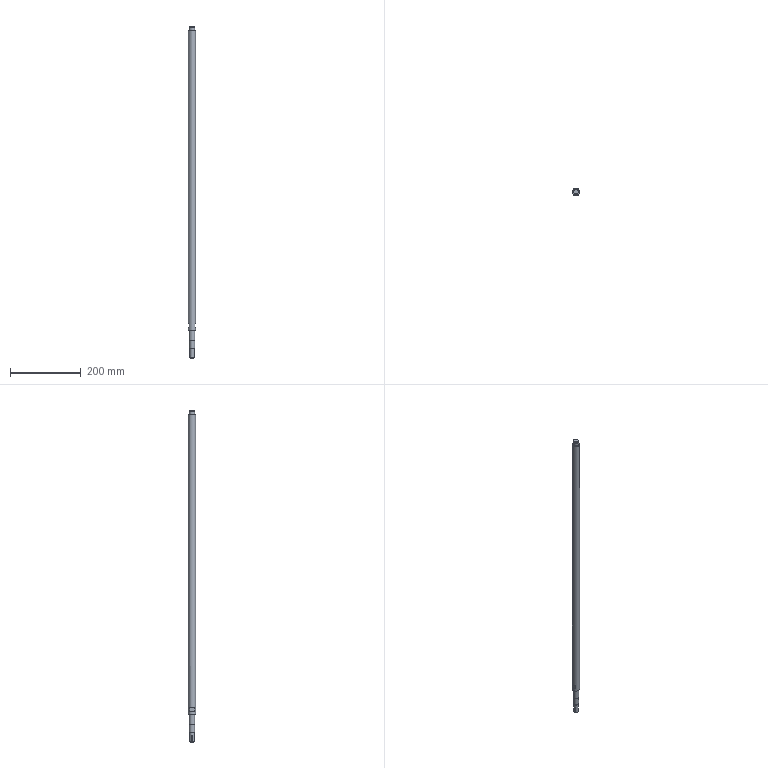Part | NX | 1 solid | 34 faces | box 20 x 20 x 936 mm | volume 278866 mm3 | plane 17 | cylinder 9 | cone 6 | torus 2 | commonest cylinder face diameters 15 x3 3.3 x1 4 x1 12 x1 14.3 x1 14.6 x1
STEP:
#1=CARTESIAN_POINT('',(7.5,0.,923.));
#2=VERTEX_POINT('',#1);
#3=CARTESIAN_POINT('',(0.,0.,923.));
#4=DIRECTION('',(0.,0.,1.));
#5=DIRECTION('',(1.,0.,0.));
#6=AXIS2_PLACEMENT_3D('',#3,#4,#5);
#7=CIRCLE('',#6,7.5);
#8=EDGE_CURVE('',#2,#2,#7,.T.);
#9=ORIENTED_EDGE('',*,*,#8,.T.);
#10=EDGE_LOOP('',(#9));
#11=FACE_BOUND('',#10,.T.);
#12=CARTESIAN_POINT('',(-7.5,0.,931.995));
#13=VERTEX_POINT('',#12);
#14=CARTESIAN_POINT('',(0.,0.,931.995));
#15=DIRECTION('',(0.,0.,-1.));
#16=DIRECTION('',(-1.,0.,0.));
#17=AXIS2_PLACEMENT_3D('',#14,#15,#16);
#18=CIRCLE('',#17,7.5);
#19=EDGE_CURVE('',#13,#13,#18,.T.);
#20=ORIENTED_EDGE('',*,*,#19,.T.);
#21=EDGE_LOOP('',(#20));
#22=FACE_BOUND('',#21,.T.);
#23=CARTESIAN_POINT('',(0.,0.,936.));
#24=DIRECTION('',(0.,0.,-1.));
#25=DIRECTION('',(-1.,0.,0.));
#26=AXIS2_PLACEMENT_3D('',#23,#24,#25);
#27=CYLINDRICAL_SURFACE('',#26,7.5);
#28=ADVANCED_FACE('',(#11,#22),#27,.T.);
#29=CARTESIAN_POINT('',(7.5,0.,78.));
#30=VERTEX_POINT('',#29);
#31=CARTESIAN_POINT('',(0.,0.,78.));
#32=DIRECTION('',(0.,0.,1.));
#33=DIRECTION('',(1.,0.,0.));
#34=AXIS2_PLACEMENT_3D('',#31,#32,#33);
#35=CIRCLE('',#34,7.5);
#36=EDGE_CURVE('',#30,#30,#35,.T.);
#37=ORIENTED_EDGE('',*,*,#36,.F.);
#38=EDGE_LOOP('',(#37));
#39=FACE_BOUND('',#38,.T.);
#40=CARTESIAN_POINT('',(-7.5,0.,50.));
#41=VERTEX_POINT('',#40);
#42=CARTESIAN_POINT('',(0.,0.,50.));
#43=DIRECTION('',(0.,0.,-1.));
#44=DIRECTION('',(-1.,0.,0.));
#45=AXIS2_PLACEMENT_3D('',#42,#43,#44);
#46=CIRCLE('',#45,7.5);
#47=EDGE_CURVE('',#41,#41,#46,.T.);
#48=ORIENTED_EDGE('',*,*,#47,.F.);
#49=EDGE_LOOP('',(#48));
#50=FACE_BOUND('',#49,.T.);
#51=CARTESIAN_POINT('',(0.,0.,78.));
#52=DIRECTION('',(0.,0.,-1.));
#53=DIRECTION('',(-1.,0.,0.));
#54=AXIS2_PLACEMENT_3D('',#51,#52,#53);
#55=CYLINDRICAL_SURFACE('',#54,7.5);
#56=ADVANCED_FACE('',(#39,#50),#55,.T.);
#57=CARTESIAN_POINT('',(10.,0.,922.7));
#58=VERTEX_POINT('',#57);
#59=CARTESIAN_POINT('',(0.,0.,922.7));
#60=DIRECTION('',(0.,0.,1.));
#61=DIRECTION('',(1.,0.,0.));
#62=AXIS2_PLACEMENT_3D('',#59,#60,#61);
#63=CIRCLE('',#62,10.);
#64=EDGE_CURVE('',#58,#58,#63,.F.);
#65=ORIENTED_EDGE('',*,*,#64,.T.);
#66=EDGE_LOOP('',(#65));
#67=FACE_BOUND('',#66,.T.);
#68=CARTESIAN_POINT('',(10.,0.,78.3));
#69=VERTEX_POINT('',#68);
#70=CARTESIAN_POINT('',(0.,0.,78.3));
#71=DIRECTION('',(0.,0.,1.));
#72=DIRECTION('',(1.,0.,0.));
#73=AXIS2_PLACEMENT_3D('',#70,#71,#72);
#74=CIRCLE('',#73,10.);
#75=EDGE_CURVE('',#69,#69,#74,.T.);
#76=ORIENTED_EDGE('',*,*,#75,.T.);
#77=EDGE_LOOP('',(#76));
#78=FACE_BOUND('',#77,.T.);
#79=CARTESIAN_POINT('',(-8.,-6.,97.));
#80=VERTEX_POINT('',#79);
#81=CARTESIAN_POINT('',(-8.,6.,97.));
#82=VERTEX_POINT('',#81);
#83=CARTESIAN_POINT('',(0.,0.,97.));
#84=DIRECTION('',(0.,0.,-1.));
#85=DIRECTION('',(-1.,0.,0.));
#86=AXIS2_PLACEMENT_3D('',#83,#84,#85);
#87=CIRCLE('',#86,10.);
#88=EDGE_CURVE('',#80,#82,#87,.T.);
#89=ORIENTED_EDGE('',*,*,#88,.F.);
#90=CARTESIAN_POINT('',(-8.,-6.,86.));
#91=VERTEX_POINT('',#90);
#92=CARTESIAN_POINT('',(-8.,-6.,923.));
#93=DIRECTION('',(0.,0.,-1.));
#94=VECTOR('',#93,1000.);
#95=LINE('',#92,#94);
#96=EDGE_CURVE('',#80,#91,#95,.T.);
#97=ORIENTED_EDGE('',*,*,#96,.T.);
#98=CARTESIAN_POINT('',(-8.,6.,86.));
#99=VERTEX_POINT('',#98);
#100=CARTESIAN_POINT('',(0.,0.,86.));
#101=DIRECTION('',(0.,0.,-1.));
#102=DIRECTION('',(-1.,0.,0.));
#103=AXIS2_PLACEMENT_3D('',#100,#101,#102);
#104=CIRCLE('',#103,10.);
#105=EDGE_CURVE('',#91,#99,#104,.T.);
#106=ORIENTED_EDGE('',*,*,#105,.T.);
#107=CARTESIAN_POINT('',(-8.,6.,923.));
#108=DIRECTION('',(0.,0.,-1.));
#109=VECTOR('',#108,1000.);
#110=LINE('',#107,#109);
#111=EDGE_CURVE('',#99,#82,#110,.F.);
#112=ORIENTED_EDGE('',*,*,#111,.T.);
#113=EDGE_LOOP('',(#89,#97,#106,#112));
#114=FACE_BOUND('',#113,.T.);
#115=CARTESIAN_POINT('',(8.,6.,97.));
#116=VERTEX_POINT('',#115);
#117=CARTESIAN_POINT('',(8.,-6.,97.));
#118=VERTEX_POINT('',#117);
#119=CARTESIAN_POINT('',(0.,0.,97.));
#120=DIRECTION('',(0.,0.,-1.));
#121=DIRECTION('',(-1.,0.,0.));
#122=AXIS2_PLACEMENT_3D('',#119,#120,#121);
#123=CIRCLE('',#122,10.);
#124=EDGE_CURVE('',#116,#118,#123,.T.);
#125=ORIENTED_EDGE('',*,*,#124,.F.);
#126=CARTESIAN_POINT('',(8.,6.,86.));
#127=VERTEX_POINT('',#126);
#128=CARTESIAN_POINT('',(8.,6.,923.));
#129=DIRECTION('',(0.,0.,-1.));
#130=VECTOR('',#129,1000.);
#131=LINE('',#128,#130);
#132=EDGE_CURVE('',#116,#127,#131,.T.);
#133=ORIENTED_EDGE('',*,*,#132,.T.);
#134=CARTESIAN_POINT('',(8.,-6.,86.));
#135=VERTEX_POINT('',#134);
#136=CARTESIAN_POINT('',(0.,0.,86.));
#137=DIRECTION('',(0.,0.,-1.));
#138=DIRECTION('',(-1.,0.,0.));
#139=AXIS2_PLACEMENT_3D('',#136,#137,#138);
#140=CIRCLE('',#139,10.);
#141=EDGE_CURVE('',#127,#135,#140,.T.);
#142=ORIENTED_EDGE('',*,*,#141,.T.);
#143=CARTESIAN_POINT('',(8.,-6.,923.));
#144=DIRECTION('',(0.,0.,-1.));
#145=VECTOR('',#144,1000.);
#146=LINE('',#143,#145);
#147=EDGE_CURVE('',#135,#118,#146,.F.);
#148=ORIENTED_EDGE('',*,*,#147,.T.);
#149=EDGE_LOOP('',(#125,#133,#142,#148));
#150=FACE_BOUND('',#149,.T.);
#151=CARTESIAN_POINT('',(0.,0.,923.));
#152=DIRECTION('',(0.,0.,-1.));
#153=DIRECTION('',(-1.,0.,0.));
#154=AXIS2_PLACEMENT_3D('',#151,#152,#153);
#155=CYLINDRICAL_SURFACE('',#154,10.);
#156=ADVANCED_FACE('',(#67,#78,#114,#150),#155,.T.);
#157=CARTESIAN_POINT('',(9.7,0.,923.));
#158=VERTEX_POINT('',#157);
#159=CARTESIAN_POINT('',(0.,0.,923.));
#160=DIRECTION('',(0.,0.,1.));
#161=DIRECTION('',(1.,0.,0.));
#162=AXIS2_PLACEMENT_3D('',#159,#160,#161);
#163=CIRCLE('',#162,9.7);
#164=EDGE_CURVE('',#158,#158,#163,.T.);
#165=ORIENTED_EDGE('',*,*,#164,.T.);
#166=EDGE_LOOP('',(#165));
#167=FACE_BOUND('',#166,.T.);
#168=ORIENTED_EDGE('',*,*,#8,.F.);
#169=EDGE_LOOP('',(#168));
#170=FACE_BOUND('',#169,.T.);
#171=CARTESIAN_POINT('',(0.,0.,923.));
#172=DIRECTION('',(0.,0.,1.));
#173=DIRECTION('',(1.,0.,0.));
#174=AXIS2_PLACEMENT_3D('',#171,#172,#173);
#175=PLANE('',#174);
#176=ADVANCED_FACE('',(#167,#170),#175,.T.);
#177=CARTESIAN_POINT('',(9.7,0.,78.));
#178=VERTEX_POINT('',#177);
#179=CARTESIAN_POINT('',(0.,0.,78.));
#180=DIRECTION('',(0.,0.,1.));
#181=DIRECTION('',(1.,0.,0.));
#182=AXIS2_PLACEMENT_3D('',#179,#180,#181);
#183=CIRCLE('',#182,9.7);
#184=EDGE_CURVE('',#178,#178,#183,.F.);
#185=ORIENTED_EDGE('',*,*,#184,.T.);
#186=EDGE_LOOP('',(#185));
#187=FACE_BOUND('',#186,.T.);
#188=ORIENTED_EDGE('',*,*,#36,.T.);
#189=EDGE_LOOP('',(#188));
#190=FACE_BOUND('',#189,.T.);
#191=CARTESIAN_POINT('',(0.,0.,78.));
#192=DIRECTION('',(0.,0.,1.));
#193=DIRECTION('',(1.,0.,0.));
#194=AXIS2_PLACEMENT_3D('',#191,#192,#193);
#195=PLANE('',#194);
#196=ADVANCED_FACE('',(#187,#190),#195,.F.);
#197=CARTESIAN_POINT('',(-8.,20.,97.));
#198=DIRECTION('',(0.,-1.,0.));
#199=VECTOR('',#198,1000.);
#200=LINE('',#197,#199);
#201=EDGE_CURVE('',#82,#80,#200,.T.);
#202=ORIENTED_EDGE('',*,*,#201,.F.);
#203=ORIENTED_EDGE('',*,*,#111,.F.);
#204=CARTESIAN_POINT('',(-8.,20.,86.));
#205=DIRECTION('',(0.,-1.,0.));
#206=VECTOR('',#205,1000.);
#207=LINE('',#204,#206);
#208=EDGE_CURVE('',#99,#91,#207,.T.);
#209=ORIENTED_EDGE('',*,*,#208,.T.);
#210=ORIENTED_EDGE('',*,*,#96,.F.);
#211=EDGE_LOOP('',(#202,#203,#209,#210));
#212=FACE_BOUND('',#211,.T.);
#213=CARTESIAN_POINT('',(-8.,20.,97.));
#214=DIRECTION('',(1.,0.,0.));
#215=DIRECTION('',(0.,0.,-1.));
#216=AXIS2_PLACEMENT_3D('',#213,#214,#215);
#217=PLANE('',#216);
#218=ADVANCED_FACE('',(#212),#217,.F.);
#219=ORIENTED_EDGE('',*,*,#88,.T.);
#220=ORIENTED_EDGE('',*,*,#201,.T.);
#221=EDGE_LOOP('',(#219,#220));
#222=FACE_BOUND('',#221,.T.);
#223=CARTESIAN_POINT('',(-20.,-20.,97.));
#224=DIRECTION('',(0.,0.,-1.));
#225=DIRECTION('',(-1.,0.,0.));
#226=AXIS2_PLACEMENT_3D('',#223,#224,#225);
#227=PLANE('',#226);
#228=ADVANCED_FACE('',(#222),#227,.T.);
#229=ORIENTED_EDGE('',*,*,#208,.F.);
#230=ORIENTED_EDGE('',*,*,#105,.F.);
#231=EDGE_LOOP('',(#229,#230));
#232=FACE_BOUND('',#231,.T.);
#233=CARTESIAN_POINT('',(-20.,-20.,86.));
#234=DIRECTION('',(0.,0.,-1.));
#235=DIRECTION('',(-1.,0.,0.));
#236=AXIS2_PLACEMENT_3D('',#233,#234,#235);
#237=PLANE('',#236);
#238=ADVANCED_FACE('',(#232),#237,.F.);
#239=CARTESIAN_POINT('',(8.,20.,97.));
#240=DIRECTION('',(0.,1.,0.));
#241=VECTOR('',#240,1000.);
#242=LINE('',#239,#241);
#243=EDGE_CURVE('',#118,#116,#242,.T.);
#244=ORIENTED_EDGE('',*,*,#243,.F.);
#245=ORIENTED_EDGE('',*,*,#147,.F.);
#246=CARTESIAN_POINT('',(8.,20.,86.));
#247=DIRECTION('',(0.,1.,0.));
#248=VECTOR('',#247,1000.);
#249=LINE('',#246,#248);
#250=EDGE_CURVE('',#135,#127,#249,.T.);
#251=ORIENTED_EDGE('',*,*,#250,.T.);
#252=ORIENTED_EDGE('',*,*,#132,.F.);
#253=EDGE_LOOP('',(#244,#245,#251,#252));
#254=FACE_BOUND('',#253,.T.);
#255=CARTESIAN_POINT('',(8.,20.,97.));
#256=DIRECTION('',(-1.,0.,0.));
#257=DIRECTION('',(0.,0.,1.));
#258=AXIS2_PLACEMENT_3D('',#255,#256,#257);
#259=PLANE('',#258);
#260=ADVANCED_FACE('',(#254),#259,.F.);
#261=ORIENTED_EDGE('',*,*,#124,.T.);
#262=ORIENTED_EDGE('',*,*,#243,.T.);
#263=EDGE_LOOP('',(#261,#262));
#264=FACE_BOUND('',#263,.T.);
#265=CARTESIAN_POINT('',(8.,-20.,97.));
#266=DIRECTION('',(0.,0.,-1.));
#267=DIRECTION('',(-1.,0.,0.));
#268=AXIS2_PLACEMENT_3D('',#265,#266,#267);
#269=PLANE('',#268);
#270=ADVANCED_FACE('',(#264),#269,.T.);
#271=ORIENTED_EDGE('',*,*,#250,.F.);
#272=ORIENTED_EDGE('',*,*,#141,.F.);
#273=EDGE_LOOP('',(#271,#272));
#274=FACE_BOUND('',#273,.T.);
#275=CARTESIAN_POINT('',(8.,-20.,86.));
#276=DIRECTION('',(0.,0.,-1.));
#277=DIRECTION('',(-1.,0.,0.));
#278=AXIS2_PLACEMENT_3D('',#275,#276,#277);
#279=PLANE('',#278);
#280=ADVANCED_FACE('',(#274),#279,.F.);
#281=ORIENTED_EDGE('',*,*,#64,.F.);
#282=EDGE_LOOP('',(#281));
#283=FACE_BOUND('',#282,.T.);
#284=ORIENTED_EDGE('',*,*,#164,.F.);
#285=EDGE_LOOP('',(#284));
#286=FACE_BOUND('',#285,.T.);
#287=CARTESIAN_POINT('',(0.,0.,923.));
#288=DIRECTION('',(0.,0.,-1.));
#289=DIRECTION('',(-1.,0.,0.));
#290=AXIS2_PLACEMENT_3D('',#287,#288,#289);
#291=CONICAL_SURFACE('',#290,9.7,0.7854);
#292=ADVANCED_FACE('',(#283,#286),#291,.T.);
#293=ORIENTED_EDGE('',*,*,#184,.F.);
#294=EDGE_LOOP('',(#293));
#295=FACE_BOUND('',#294,.T.);
#296=ORIENTED_EDGE('',*,*,#75,.F.);
#297=EDGE_LOOP('',(#296));
#298=FACE_BOUND('',#297,.T.);
#299=CARTESIAN_POINT('',(0.,0.,78.3));
#300=DIRECTION('',(0.,0.,1.));
#301=DIRECTION('',(1.,0.,0.));
#302=AXIS2_PLACEMENT_3D('',#299,#300,#301);
#303=CONICAL_SURFACE('',#302,10.,0.7854);
#304=ADVANCED_FACE('',(#295,#298),#303,.T.);
#305=CARTESIAN_POINT('',(-7.3,0.,50.));
#306=VERTEX_POINT('',#305);
#307=CARTESIAN_POINT('',(0.,0.,50.));
#308=DIRECTION('',(0.,0.,-1.));
#309=DIRECTION('',(-1.,0.,0.));
#310=AXIS2_PLACEMENT_3D('',#307,#308,#309);
#311=CIRCLE('',#310,7.3);
#312=EDGE_CURVE('',#306,#306,#311,.T.);
#313=ORIENTED_EDGE('',*,*,#312,.F.);
#314=EDGE_LOOP('',(#313));
#315=FACE_BOUND('',#314,.T.);
#316=ORIENTED_EDGE('',*,*,#47,.T.);
#317=EDGE_LOOP('',(#316));
#318=FACE_BOUND('',#317,.T.);
#319=CARTESIAN_POINT('',(0.,0.,50.));
#320=DIRECTION('',(0.,0.,-1.));
#321=DIRECTION('',(-1.,0.,0.));
#322=AXIS2_PLACEMENT_3D('',#319,#320,#321);
#323=PLANE('',#322);
#324=ADVANCED_FACE('',(#315,#318),#323,.T.);
#325=CARTESIAN_POINT('',(7.3,0.,28.1));
#326=VERTEX_POINT('',#325);
#327=CARTESIAN_POINT('',(0.,0.,28.1));
#328=DIRECTION('',(0.,0.,1.));
#329=DIRECTION('',(1.,0.,0.));
#330=AXIS2_PLACEMENT_3D('',#327,#328,#329);
#331=CIRCLE('',#330,7.3);
#332=EDGE_CURVE('',#326,#326,#331,.F.);
#333=ORIENTED_EDGE('',*,*,#332,.F.);
#334=EDGE_LOOP('',(#333));
#335=FACE_BOUND('',#334,.T.);
#336=ORIENTED_EDGE('',*,*,#312,.T.);
#337=EDGE_LOOP('',(#336));
#338=FACE_BOUND('',#337,.T.);
#339=CARTESIAN_POINT('',(0.,0.,50.));
#340=DIRECTION('',(0.,0.,-1.));
#341=DIRECTION('',(-1.,0.,0.));
#342=AXIS2_PLACEMENT_3D('',#339,#340,#341);
#343=CYLINDRICAL_SURFACE('',#342,7.3);
#344=ADVANCED_FACE('',(#335,#338),#343,.T.);
#345=CARTESIAN_POINT('',(-1.65,0.,0.));
#346=VERTEX_POINT('',#345);
#347=CARTESIAN_POINT('',(0.,0.,0.));
#348=DIRECTION('',(0.,0.,-1.));
#349=DIRECTION('',(-1.,0.,0.));
#350=AXIS2_PLACEMENT_3D('',#347,#348,#349);
#351=CIRCLE('',#350,1.65);
#352=EDGE_CURVE('',#346,#346,#351,.T.);
#353=ORIENTED_EDGE('',*,*,#352,.F.);
#354=EDGE_LOOP('',(#353));
#355=FACE_BOUND('',#354,.T.);
#356=CARTESIAN_POINT('',(-3.5,2.,0.));
#357=VERTEX_POINT('',#356);
#358=CARTESIAN_POINT('',(-3.5,-2.,0.));
#359=VERTEX_POINT('',#358);
#360=CARTESIAN_POINT('',(-3.5,0.,0.));
#361=DIRECTION('',(0.,-1.,0.));
#362=VECTOR('',#361,1000.);
#363=LINE('',#360,#362);
#364=EDGE_CURVE('',#357,#359,#363,.T.);
#365=ORIENTED_EDGE('',*,*,#364,.F.);
#366=CARTESIAN_POINT('',(-4.583,2.,0.));
#367=VERTEX_POINT('',#366);
#368=CARTESIAN_POINT('',(-3.5,2.,0.));
#369=DIRECTION('',(-1.,0.,0.));
#370=VECTOR('',#369,1000.);
#371=LINE('',#368,#370);
#372=EDGE_CURVE('',#357,#367,#371,.T.);
#373=ORIENTED_EDGE('',*,*,#372,.T.);
#374=CARTESIAN_POINT('',(-4.583,-2.,0.));
#375=VERTEX_POINT('',#374);
#376=CARTESIAN_POINT('',(0.,0.,0.));
#377=DIRECTION('',(0.,0.,1.));
#378=DIRECTION('',(1.,0.,0.));
#379=AXIS2_PLACEMENT_3D('',#376,#377,#378);
#380=CIRCLE('',#379,5.);
#381=EDGE_CURVE('',#367,#375,#380,.F.);
#382=ORIENTED_EDGE('',*,*,#381,.T.);
#383=CARTESIAN_POINT('',(-3.5,-2.,0.));
#384=DIRECTION('',(-1.,0.,0.));
#385=VECTOR('',#384,1000.);
#386=LINE('',#383,#385);
#387=EDGE_CURVE('',#359,#375,#386,.T.);
#388=ORIENTED_EDGE('',*,*,#387,.F.);
#389=EDGE_LOOP('',(#365,#373,#382,#388));
#390=FACE_BOUND('',#389,.T.);
#391=CARTESIAN_POINT('',(0.,0.,0.));
#392=DIRECTION('',(0.,0.,1.));
#393=DIRECTION('',(1.,0.,0.));
#394=AXIS2_PLACEMENT_3D('',#391,#392,#393);
#395=PLANE('',#394);
#396=ADVANCED_FACE('',(#355,#390),#395,.F.);
#397=CARTESIAN_POINT('',(-5.657,-2.,1.));
#398=VERTEX_POINT('',#397);
#399=CARTESIAN_POINT('',(-5.657,2.,1.));
#400=VERTEX_POINT('',#399);
#401=CARTESIAN_POINT('',(0.,0.,1.));
#402=DIRECTION('',(0.,0.,1.));
#403=DIRECTION('',(1.,0.,0.));
#404=AXIS2_PLACEMENT_3D('',#401,#402,#403);
#405=CIRCLE('',#404,6.);
#406=EDGE_CURVE('',#398,#400,#405,.T.);
#407=ORIENTED_EDGE('',*,*,#406,.T.);
#408=CARTESIAN_POINT('',(-5.657,2.,16.));
#409=VERTEX_POINT('',#408);
#410=CARTESIAN_POINT('',(-5.657,2.,28.));
#411=DIRECTION('',(0.,0.,-1.));
#412=VECTOR('',#411,1000.);
#413=LINE('',#410,#412);
#414=EDGE_CURVE('',#400,#409,#413,.F.);
#415=ORIENTED_EDGE('',*,*,#414,.T.);
#416=CARTESIAN_POINT('',(-5.657,-2.,16.));
#417=VERTEX_POINT('',#416);
#418=CARTESIAN_POINT('',(-5.657,2.,16.));
#419=CARTESIAN_POINT('',(-5.657,2.,16.533));
#420=CARTESIAN_POINT('',(-5.833,1.567,17.562));
#421=CARTESIAN_POINT('',(-6.083,0.003461,18.219));
#422=CARTESIAN_POINT('',(-5.834,-1.568,17.563));
#423=CARTESIAN_POINT('',(-5.657,-2.,16.533));
#424=CARTESIAN_POINT('',(-5.657,-2.,16.));
#425=B_SPLINE_CURVE_WITH_KNOTS('',3,(#418,#419,#420,#421,#422,#423,#424),.UNSPECIFIED.,.F.,.F.,(4,1,1,1,4),(0.,0.001574,0.003148,0.004722,0.006296),.UNSPECIFIED.);
#426=EDGE_CURVE('',#409,#417,#425,.T.);
#427=ORIENTED_EDGE('',*,*,#426,.T.);
#428=CARTESIAN_POINT('',(-5.657,-2.,28.));
#429=DIRECTION('',(0.,0.,-1.));
#430=VECTOR('',#429,1000.);
#431=LINE('',#428,#430);
#432=EDGE_CURVE('',#417,#398,#431,.T.);
#433=ORIENTED_EDGE('',*,*,#432,.T.);
#434=EDGE_LOOP('',(#407,#415,#427,#433));
#435=FACE_BOUND('',#434,.T.);
#436=CARTESIAN_POINT('',(6.,0.,28.));
#437=VERTEX_POINT('',#436);
#438=CARTESIAN_POINT('',(0.,0.,28.));
#439=DIRECTION('',(0.,0.,1.));
#440=DIRECTION('',(1.,0.,0.));
#441=AXIS2_PLACEMENT_3D('',#438,#439,#440);
#442=CIRCLE('',#441,6.);
#443=EDGE_CURVE('',#437,#437,#442,.T.);
#444=ORIENTED_EDGE('',*,*,#443,.F.);
#445=EDGE_LOOP('',(#444));
#446=FACE_BOUND('',#445,.T.);
#447=CARTESIAN_POINT('',(0.,0.,28.));
#448=DIRECTION('',(0.,0.,-1.));
#449=DIRECTION('',(-1.,0.,0.));
#450=AXIS2_PLACEMENT_3D('',#447,#448,#449);
#451=CYLINDRICAL_SURFACE('',#450,6.);
#452=ADVANCED_FACE('',(#435,#446),#451,.T.);
#453=CARTESIAN_POINT('',(7.2,0.,28.));
#454=VERTEX_POINT('',#453);
#455=CARTESIAN_POINT('',(0.,0.,28.));
#456=DIRECTION('',(0.,0.,1.));
#457=DIRECTION('',(1.,0.,0.));
#458=AXIS2_PLACEMENT_3D('',#455,#456,#457);
#459=CIRCLE('',#458,7.2);
#460=EDGE_CURVE('',#454,#454,#459,.F.);
#461=ORIENTED_EDGE('',*,*,#460,.T.);
#462=EDGE_LOOP('',(#461));
#463=FACE_BOUND('',#462,.T.);
#464=ORIENTED_EDGE('',*,*,#443,.T.);
#465=EDGE_LOOP('',(#464));
#466=FACE_BOUND('',#465,.T.);
#467=CARTESIAN_POINT('',(0.,0.,28.));
#468=DIRECTION('',(0.,0.,1.));
#469=DIRECTION('',(1.,0.,0.));
#470=AXIS2_PLACEMENT_3D('',#467,#468,#469);
#471=PLANE('',#470);
#472=ADVANCED_FACE('',(#463,#466),#471,.F.);
#473=ORIENTED_EDGE('',*,*,#460,.F.);
#474=EDGE_LOOP('',(#473));
#475=FACE_BOUND('',#474,.T.);
#476=ORIENTED_EDGE('',*,*,#332,.T.);
#477=EDGE_LOOP('',(#476));
#478=FACE_BOUND('',#477,.T.);
#479=CARTESIAN_POINT('',(0.,0.,28.3));
#480=DIRECTION('',(0.,0.,1.));
#481=DIRECTION('',(1.,0.,0.));
#482=AXIS2_PLACEMENT_3D('',#479,#480,#481);
#483=CONICAL_SURFACE('',#482,7.5,0.7854);
#484=ADVANCED_FACE('',(#475,#478),#483,.T.);
#485=CARTESIAN_POINT('',(-7.5,0.,933.145));
#486=VERTEX_POINT('',#485);
#487=CARTESIAN_POINT('',(0.,0.,933.145));
#488=DIRECTION('',(0.,0.,-1.));
#489=DIRECTION('',(-1.,0.,0.));
#490=AXIS2_PLACEMENT_3D('',#487,#488,#489);
#491=CIRCLE('',#490,7.5);
#492=EDGE_CURVE('',#486,#486,#491,.T.);
#493=ORIENTED_EDGE('',*,*,#492,.T.);
#494=EDGE_LOOP('',(#493));
#495=FACE_BOUND('',#494,.T.);
#496=CARTESIAN_POINT('',(-7.26,0.,933.145));
#497=VERTEX_POINT('',#496);
#498=CARTESIAN_POINT('',(0.,0.,933.145));
#499=DIRECTION('',(0.,0.,-1.));
#500=DIRECTION('',(-1.,0.,0.));
#501=AXIS2_PLACEMENT_3D('',#498,#499,#500);
#502=CIRCLE('',#501,7.26);
#503=EDGE_CURVE('',#497,#497,#502,.T.);
#504=ORIENTED_EDGE('',*,*,#503,.F.);
#505=EDGE_LOOP('',(#504));
#506=FACE_BOUND('',#505,.T.);
#507=CARTESIAN_POINT('',(-7.26,-0.05092,933.145));
#508=DIRECTION('',(0.,0.,-1.));
#509=DIRECTION('',(-1.,0.,0.));
#510=AXIS2_PLACEMENT_3D('',#507,#508,#509);
#511=PLANE('',#510);
#512=ADVANCED_FACE('',(#495,#506),#511,.T.);
#513=ORIENTED_EDGE('',*,*,#503,.T.);
#514=EDGE_LOOP('',(#513));
#515=FACE_BOUND('',#514,.T.);
#516=CARTESIAN_POINT('',(-7.15,0.,933.035));
#517=VERTEX_POINT('',#516);
#518=CARTESIAN_POINT('',(0.,0.,933.035));
#519=DIRECTION('',(0.,0.,-1.));
#520=DIRECTION('',(-1.,0.,0.));
#521=AXIS2_PLACEMENT_3D('',#518,#519,#520);
#522=CIRCLE('',#521,7.15);
#523=EDGE_CURVE('',#517,#517,#522,.T.);
#524=ORIENTED_EDGE('',*,*,#523,.F.);
#525=EDGE_LOOP('',(#524));
#526=FACE_BOUND('',#525,.T.);
#527=CARTESIAN_POINT('',(0.,0.,933.035));
#528=DIRECTION('',(0.,0.,-1.));
#529=DIRECTION('',(-1.,0.,0.));
#530=AXIS2_PLACEMENT_3D('',#527,#528,#529);
#531=TOROIDAL_SURFACE('',#530,7.26,0.11);
#532=ADVANCED_FACE('',(#515,#526),#531,.F.);
#533=ORIENTED_EDGE('',*,*,#523,.T.);
#534=EDGE_LOOP('',(#533));
#535=FACE_BOUND('',#534,.T.);
#536=CARTESIAN_POINT('',(-7.15,0.,932.105));
#537=VERTEX_POINT('',#536);
#538=CARTESIAN_POINT('',(0.,0.,932.105));
#539=DIRECTION('',(0.,0.,-1.));
#540=DIRECTION('',(-1.,0.,0.));
#541=AXIS2_PLACEMENT_3D('',#538,#539,#540);
#542=CIRCLE('',#541,7.15);
#543=EDGE_CURVE('',#537,#537,#542,.T.);
#544=ORIENTED_EDGE('',*,*,#543,.F.);
#545=EDGE_LOOP('',(#544));
#546=FACE_BOUND('',#545,.T.);
#547=CARTESIAN_POINT('',(0.,0.,1053.848));
#548=DIRECTION('',(0.,0.,-1.));
#549=DIRECTION('',(-1.,0.,0.));
#550=AXIS2_PLACEMENT_3D('',#547,#548,#549);
#551=CYLINDRICAL_SURFACE('',#550,7.15);
#552=ADVANCED_FACE('',(#535,#546),#551,.T.);
#553=ORIENTED_EDGE('',*,*,#543,.T.);
#554=EDGE_LOOP('',(#553));
#555=FACE_BOUND('',#554,.T.);
#556=CARTESIAN_POINT('',(-7.26,0.,931.995));
#557=VERTEX_POINT('',#556);
#558=CARTESIAN_POINT('',(0.,0.,931.995));
#559=DIRECTION('',(0.,0.,-1.));
#560=DIRECTION('',(-1.,0.,0.));
#561=AXIS2_PLACEMENT_3D('',#558,#559,#560);
#562=CIRCLE('',#561,7.26);
#563=EDGE_CURVE('',#557,#557,#562,.T.);
#564=ORIENTED_EDGE('',*,*,#563,.F.);
#565=EDGE_LOOP('',(#564));
#566=FACE_BOUND('',#565,.T.);
#567=CARTESIAN_POINT('',(0.,0.,932.105));
#568=DIRECTION('',(0.,0.,-1.));
#569=DIRECTION('',(-1.,0.,0.));
#570=AXIS2_PLACEMENT_3D('',#567,#568,#569);
#571=TOROIDAL_SURFACE('',#570,7.26,0.11);
#572=ADVANCED_FACE('',(#555,#566),#571,.F.);
#573=ORIENTED_EDGE('',*,*,#563,.T.);
#574=EDGE_LOOP('',(#573));
#575=FACE_BOUND('',#574,.T.);
#576=ORIENTED_EDGE('',*,*,#19,.F.);
#577=EDGE_LOOP('',(#576));
#578=FACE_BOUND('',#577,.T.);
#579=CARTESIAN_POINT('',(-7.5,-0.0526,931.995));
#580=DIRECTION('',(0.,0.,1.));
#581=DIRECTION('',(1.,0.,0.));
#582=AXIS2_PLACEMENT_3D('',#579,#580,#581);
#583=PLANE('',#582);
#584=ADVANCED_FACE('',(#575,#578),#583,.T.);
#585=CARTESIAN_POINT('',(6.5,0.,936.));
#586=VERTEX_POINT('',#585);
#587=CARTESIAN_POINT('',(0.,0.,936.));
#588=DIRECTION('',(0.,0.,1.));
#589=DIRECTION('',(1.,0.,0.));
#590=AXIS2_PLACEMENT_3D('',#587,#588,#589);
#591=CIRCLE('',#590,6.5);
#592=EDGE_CURVE('',#586,#586,#591,.T.);
#593=ORIENTED_EDGE('',*,*,#592,.T.);
#594=EDGE_LOOP('',(#593));
#595=FACE_BOUND('',#594,.T.);
#596=CARTESIAN_POINT('',(0.,0.,936.));
#597=DIRECTION('',(0.,0.,1.));
#598=DIRECTION('',(1.,0.,0.));
#599=AXIS2_PLACEMENT_3D('',#596,#597,#598);
#600=PLANE('',#599);
#601=ADVANCED_FACE('',(#595),#600,.T.);
#602=CARTESIAN_POINT('',(7.5,0.,935.));
#603=VERTEX_POINT('',#602);
#604=CARTESIAN_POINT('',(0.,0.,935.));
#605=DIRECTION('',(0.,0.,1.));
#606=DIRECTION('',(1.,0.,0.));
#607=AXIS2_PLACEMENT_3D('',#604,#605,#606);
#608=CIRCLE('',#607,7.5);
#609=EDGE_CURVE('',#603,#603,#608,.F.);
#610=ORIENTED_EDGE('',*,*,#609,.T.);
#611=EDGE_LOOP('',(#610));
#612=FACE_BOUND('',#611,.T.);
#613=ORIENTED_EDGE('',*,*,#492,.F.);
#614=EDGE_LOOP('',(#613));
#615=FACE_BOUND('',#614,.T.);
#616=CARTESIAN_POINT('',(0.,0.,936.));
#617=DIRECTION('',(0.,0.,-1.));
#618=DIRECTION('',(-1.,0.,0.));
#619=AXIS2_PLACEMENT_3D('',#616,#617,#618);
#620=CYLINDRICAL_SURFACE('',#619,7.5);
#621=ADVANCED_FACE('',(#612,#615),#620,.T.);
#622=ORIENTED_EDGE('',*,*,#609,.F.);
#623=EDGE_LOOP('',(#622));
#624=FACE_BOUND('',#623,.T.);
#625=ORIENTED_EDGE('',*,*,#592,.F.);
#626=EDGE_LOOP('',(#625));
#627=FACE_BOUND('',#626,.T.);
#628=CARTESIAN_POINT('',(0.,0.,936.));
#629=DIRECTION('',(0.,0.,-1.));
#630=DIRECTION('',(-1.,0.,0.));
#631=AXIS2_PLACEMENT_3D('',#628,#629,#630);
#632=CONICAL_SURFACE('',#631,6.5,0.7854);
#633=ADVANCED_FACE('',(#624,#627),#632,.T.);
#634=CARTESIAN_POINT('',(-5.657,2.,1.));
#635=CARTESIAN_POINT('',(-5.301,2.,0.6643));
#636=CARTESIAN_POINT('',(-4.943,2.,0.3304));
#637=CARTESIAN_POINT('',(-4.583,2.,0.));
#638=B_SPLINE_CURVE_WITH_KNOTS('',3,(#634,#635,#636,#637),.UNSPECIFIED.,.F.,.F.,(4,4),(0.005088,0.006556),.UNSPECIFIED.);
#639=EDGE_CURVE('',#400,#367,#638,.T.);
#640=ORIENTED_EDGE('',*,*,#639,.F.);
#641=ORIENTED_EDGE('',*,*,#406,.F.);
#642=CARTESIAN_POINT('',(-4.583,-2.,0.));
#643=CARTESIAN_POINT('',(-4.943,-2.,0.3305));
#644=CARTESIAN_POINT('',(-5.301,-2.,0.6644));
#645=CARTESIAN_POINT('',(-5.657,-2.,1.));
#646=B_SPLINE_CURVE_WITH_KNOTS('',3,(#642,#643,#644,#645),.UNSPECIFIED.,.F.,.F.,(4,4),(0.004277,0.005741),.UNSPECIFIED.);
#647=EDGE_CURVE('',#375,#398,#646,.T.);
#648=ORIENTED_EDGE('',*,*,#647,.F.);
#649=ORIENTED_EDGE('',*,*,#381,.F.);
#650=EDGE_LOOP('',(#640,#641,#648,#649));
#651=FACE_BOUND('',#650,.T.);
#652=CARTESIAN_POINT('',(0.,0.,1.));
#653=DIRECTION('',(0.,0.,1.));
#654=DIRECTION('',(1.,0.,0.));
#655=AXIS2_PLACEMENT_3D('',#652,#653,#654);
#656=CONICAL_SURFACE('',#655,6.,0.7854);
#657=ADVANCED_FACE('',(#651),#656,.T.);
#658=ORIENTED_EDGE('',*,*,#364,.T.);
#659=CARTESIAN_POINT('',(-3.5,-2.,16.));
#660=VERTEX_POINT('',#659);
#661=CARTESIAN_POINT('',(-3.5,-2.,0.));
#662=DIRECTION('',(0.,0.,1.));
#663=VECTOR('',#662,1000.);
#664=LINE('',#661,#663);
#665=EDGE_CURVE('',#359,#660,#664,.T.);
#666=ORIENTED_EDGE('',*,*,#665,.T.);
#667=CARTESIAN_POINT('',(-3.5,2.,16.));
#668=VERTEX_POINT('',#667);
#669=CARTESIAN_POINT('',(-3.5,0.,16.));
#670=DIRECTION('',(-1.,0.,0.));
#671=DIRECTION('',(0.,0.,1.));
#672=AXIS2_PLACEMENT_3D('',#669,#670,#671);
#673=CIRCLE('',#672,2.);
#674=EDGE_CURVE('',#660,#668,#673,.T.);
#675=ORIENTED_EDGE('',*,*,#674,.T.);
#676=CARTESIAN_POINT('',(-3.5,2.,0.));
#677=DIRECTION('',(0.,0.,-1.));
#678=VECTOR('',#677,1000.);
#679=LINE('',#676,#678);
#680=EDGE_CURVE('',#668,#357,#679,.T.);
#681=ORIENTED_EDGE('',*,*,#680,.T.);
#682=EDGE_LOOP('',(#658,#666,#675,#681));
#683=FACE_BOUND('',#682,.T.);
#684=CARTESIAN_POINT('',(-3.5,0.,0.));
#685=DIRECTION('',(-1.,0.,0.));
#686=DIRECTION('',(0.,0.,1.));
#687=AXIS2_PLACEMENT_3D('',#684,#685,#686);
#688=PLANE('',#687);
#689=ADVANCED_FACE('',(#683),#688,.T.);
#690=CARTESIAN_POINT('',(-3.5,2.,16.));
#691=DIRECTION('',(-1.,0.,0.));
#692=VECTOR('',#691,1000.);
#693=LINE('',#690,#692);
#694=EDGE_CURVE('',#668,#409,#693,.T.);
#695=ORIENTED_EDGE('',*,*,#694,.F.);
#696=ORIENTED_EDGE('',*,*,#674,.F.);
#697=CARTESIAN_POINT('',(-3.5,-2.,16.));
#698=DIRECTION('',(-1.,0.,0.));
#699=VECTOR('',#698,1000.);
#700=LINE('',#697,#699);
#701=EDGE_CURVE('',#660,#417,#700,.T.);
#702=ORIENTED_EDGE('',*,*,#701,.T.);
#703=ORIENTED_EDGE('',*,*,#426,.F.);
#704=EDGE_LOOP('',(#695,#696,#702,#703));
#705=FACE_BOUND('',#704,.T.);
#706=CARTESIAN_POINT('',(-3.5,0.,16.));
#707=DIRECTION('',(-1.,0.,0.));
#708=DIRECTION('',(0.,0.,1.));
#709=AXIS2_PLACEMENT_3D('',#706,#707,#708);
#710=CYLINDRICAL_SURFACE('',#709,2.);
#711=ADVANCED_FACE('',(#705),#710,.F.);
#712=ORIENTED_EDGE('',*,*,#639,.T.);
#713=ORIENTED_EDGE('',*,*,#372,.F.);
#714=ORIENTED_EDGE('',*,*,#680,.F.);
#715=ORIENTED_EDGE('',*,*,#694,.T.);
#716=ORIENTED_EDGE('',*,*,#414,.F.);
#717=EDGE_LOOP('',(#712,#713,#714,#715,#716));
#718=FACE_BOUND('',#717,.T.);
#719=CARTESIAN_POINT('',(-3.5,2.,0.));
#720=DIRECTION('',(0.,1.,0.));
#721=DIRECTION('',(0.,0.,1.));
#722=AXIS2_PLACEMENT_3D('',#719,#720,#721);
#723=PLANE('',#722);
#724=ADVANCED_FACE('',(#718),#723,.F.);
#725=ORIENTED_EDGE('',*,*,#701,.F.);
#726=ORIENTED_EDGE('',*,*,#665,.F.);
#727=ORIENTED_EDGE('',*,*,#387,.T.);
#728=ORIENTED_EDGE('',*,*,#647,.T.);
#729=ORIENTED_EDGE('',*,*,#432,.F.);
#730=EDGE_LOOP('',(#725,#726,#727,#728,#729));
#731=FACE_BOUND('',#730,.T.);
#732=CARTESIAN_POINT('',(-3.5,-2.,0.));
#733=DIRECTION('',(0.,-1.,0.));
#734=DIRECTION('',(0.,0.,-1.));
#735=AXIS2_PLACEMENT_3D('',#732,#733,#734);
#736=PLANE('',#735);
#737=ADVANCED_FACE('',(#731),#736,.F.);
#738=CARTESIAN_POINT('',(0.,0.,12.491));
#739=VERTEX_POINT('',#738);
#740=VERTEX_LOOP('',#739);
#741=FACE_BOUND('',#740,.T.);
#742=CARTESIAN_POINT('',(-1.65,0.,11.5));
#743=VERTEX_POINT('',#742);
#744=CARTESIAN_POINT('',(0.,0.,11.5));
#745=DIRECTION('',(0.,0.,-1.));
#746=DIRECTION('',(-1.,0.,0.));
#747=AXIS2_PLACEMENT_3D('',#744,#745,#746);
#748=CIRCLE('',#747,1.65);
#749=EDGE_CURVE('',#743,#743,#748,.T.);
#750=ORIENTED_EDGE('',*,*,#749,.T.);
#751=EDGE_LOOP('',(#750));
#752=FACE_BOUND('',#751,.T.);
#753=CARTESIAN_POINT('',(0.,0.,11.5));
#754=DIRECTION('',(0.,0.,-1.));
#755=DIRECTION('',(-1.,0.,0.));
#756=AXIS2_PLACEMENT_3D('',#753,#754,#755);
#757=CONICAL_SURFACE('',#756,1.65,1.03);
#758=ADVANCED_FACE('',(#741,#752),#757,.F.);
#759=ORIENTED_EDGE('',*,*,#749,.F.);
#760=EDGE_LOOP('',(#759));
#761=FACE_BOUND('',#760,.T.);
#762=ORIENTED_EDGE('',*,*,#352,.T.);
#763=EDGE_LOOP('',(#762));
#764=FACE_BOUND('',#763,.T.);
#765=CARTESIAN_POINT('',(0.,0.,0.));
#766=DIRECTION('',(0.,0.,-1.));
#767=DIRECTION('',(-1.,0.,0.));
#768=AXIS2_PLACEMENT_3D('',#765,#766,#767);
#769=CYLINDRICAL_SURFACE('',#768,1.65);
#770=ADVANCED_FACE('',(#761,#764),#769,.F.);
#771=CLOSED_SHELL('',(#28,#56,#156,#176,#196,#218,#228,#238,#260,#270,#280,#292,#304,#324,#344,#396,#452,#472,#484,#512,#532,#552,#572,#584,#601,#621,#633,#657,#689,#711,#724,#737,#758,#770));
#772=MANIFOLD_SOLID_BREP('',#771);
#773=(LENGTH_UNIT()NAMED_UNIT(*)SI_UNIT(.MILLI.,.METRE.));
#774=UNCERTAINTY_MEASURE_WITH_UNIT(LENGTH_MEASURE(0.0508),#773,'','');
#775=(NAMED_UNIT(*)PLANE_ANGLE_UNIT()SI_UNIT($,.RADIAN.));
#776=(NAMED_UNIT(*)SI_UNIT($,.STERADIAN.)SOLID_ANGLE_UNIT());
#777=(GEOMETRIC_REPRESENTATION_CONTEXT(3)GLOBAL_UNCERTAINTY_ASSIGNED_CONTEXT((#774))GLOBAL_UNIT_ASSIGNED_CONTEXT((#773,#775,#776))REPRESENTATION_CONTEXT('',''));
#778=ADVANCED_BREP_SHAPE_REPRESENTATION('',(#772),#777);